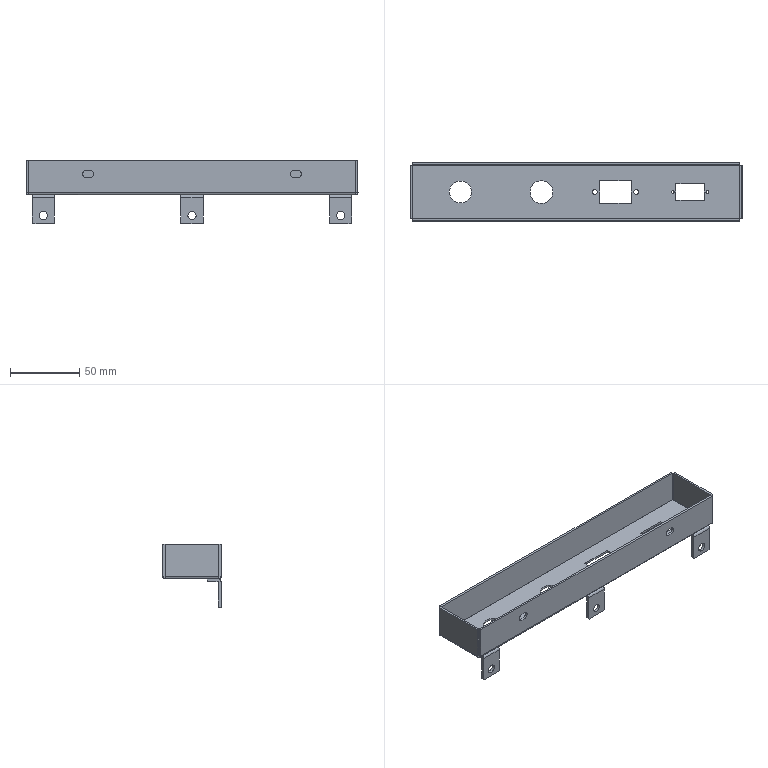Part | NX | features BREP 4 | 4 solids | 108 faces | box 240 x 42 x 46 mm | volume 35124 mm3 | plane 64 | cylinder 36 | spline 8 | commonest cylinder face diameters 6 x6 0.02 x4 2.05 x4 3.02 x4 3.5 x4 5 x4